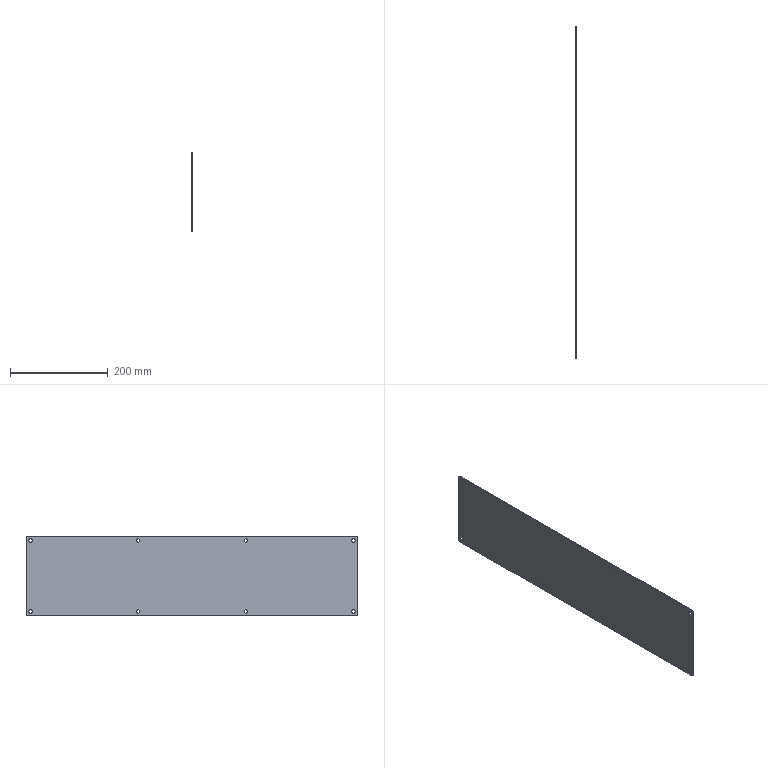Part | NX | features solid 2 | 1 solid | 26 faces | box 1.5 x 678 x 163 mm | volume 165289 mm3 | cylinder 20 | plane 6 | commonest cylinder face diameters 7 x16 8 x4
STEP:
#1=CARTESIAN_POINT('',(-1101.5,-560.,-226.5));
#2=VERTEX_POINT('',#1);
#3=CARTESIAN_POINT('',(-1100.,-560.,-226.5));
#4=VERTEX_POINT('',#3);
#5=CARTESIAN_POINT('',(-404.18,-560.,-226.5));
#6=DIRECTION('',(-1.,0.,0.));
#7=VECTOR('',#6,1000.);
#8=LINE('',#5,#7);
#9=EDGE_CURVE('',#2,#4,#8,.F.);
#10=ORIENTED_EDGE('',*,*,#9,.T.);
#11=CARTESIAN_POINT('',(-1100.,-560.,-233.5));
#12=VERTEX_POINT('',#11);
#13=CARTESIAN_POINT('',(-1100.,-560.,-230.));
#14=DIRECTION('',(-1.,0.,0.));
#15=DIRECTION('',(0.,0.,-1.));
#16=AXIS2_PLACEMENT_3D('',#13,#14,#15);
#17=CIRCLE('',#16,3.5);
#18=EDGE_CURVE('',#12,#4,#17,.T.);
#19=ORIENTED_EDGE('',*,*,#18,.F.);
#20=CARTESIAN_POINT('',(-1101.5,-560.,-233.5));
#21=VERTEX_POINT('',#20);
#22=CARTESIAN_POINT('',(-404.18,-560.,-233.5));
#23=DIRECTION('',(-1.,0.,0.));
#24=VECTOR('',#23,1000.);
#25=LINE('',#22,#24);
#26=EDGE_CURVE('',#12,#21,#25,.T.);
#27=ORIENTED_EDGE('',*,*,#26,.T.);
#28=CARTESIAN_POINT('',(-1101.5,-560.,-230.));
#29=DIRECTION('',(-1.,0.,0.));
#30=DIRECTION('',(0.,-1.,0.));
#31=AXIS2_PLACEMENT_3D('',#28,#29,#30);
#32=CIRCLE('',#31,3.5);
#33=EDGE_CURVE('',#21,#2,#32,.T.);
#34=ORIENTED_EDGE('',*,*,#33,.T.);
#35=EDGE_LOOP('',(#10,#19,#27,#34));
#36=FACE_BOUND('',#35,.T.);
#37=CARTESIAN_POINT('',(-404.18,-560.,-230.));
#38=DIRECTION('',(-1.,0.,0.));
#39=DIRECTION('',(0.,0.,-1.));
#40=AXIS2_PLACEMENT_3D('',#37,#38,#39);
#41=CYLINDRICAL_SURFACE('',#40,3.5);
#42=ADVANCED_FACE('',(#36),#41,.F.);
#43=CARTESIAN_POINT('',(-1100.,-340.,-226.5));
#44=VERTEX_POINT('',#43);
#45=CARTESIAN_POINT('',(-1101.5,-340.,-226.5));
#46=VERTEX_POINT('',#45);
#47=CARTESIAN_POINT('',(-404.18,-340.,-226.5));
#48=DIRECTION('',(-1.,0.,0.));
#49=VECTOR('',#48,1000.);
#50=LINE('',#47,#49);
#51=EDGE_CURVE('',#44,#46,#50,.T.);
#52=ORIENTED_EDGE('',*,*,#51,.F.);
#53=CARTESIAN_POINT('',(-1100.,-340.,-233.5));
#54=VERTEX_POINT('',#53);
#55=CARTESIAN_POINT('',(-1100.,-340.,-230.));
#56=DIRECTION('',(-1.,0.,0.));
#57=DIRECTION('',(0.,0.,-1.));
#58=AXIS2_PLACEMENT_3D('',#55,#56,#57);
#59=CIRCLE('',#58,3.5);
#60=EDGE_CURVE('',#54,#44,#59,.T.);
#61=ORIENTED_EDGE('',*,*,#60,.F.);
#62=CARTESIAN_POINT('',(-1101.5,-340.,-233.5));
#63=VERTEX_POINT('',#62);
#64=CARTESIAN_POINT('',(-404.18,-340.,-233.5));
#65=DIRECTION('',(-1.,0.,0.));
#66=VECTOR('',#65,1000.);
#67=LINE('',#64,#66);
#68=EDGE_CURVE('',#63,#54,#67,.F.);
#69=ORIENTED_EDGE('',*,*,#68,.F.);
#70=CARTESIAN_POINT('',(-1101.5,-340.,-230.));
#71=DIRECTION('',(-1.,0.,0.));
#72=DIRECTION('',(0.,-1.,0.));
#73=AXIS2_PLACEMENT_3D('',#70,#71,#72);
#74=CIRCLE('',#73,3.5);
#75=EDGE_CURVE('',#63,#46,#74,.T.);
#76=ORIENTED_EDGE('',*,*,#75,.T.);
#77=EDGE_LOOP('',(#52,#61,#69,#76));
#78=FACE_BOUND('',#77,.T.);
#79=CARTESIAN_POINT('',(-404.18,-340.,-230.));
#80=DIRECTION('',(-1.,0.,0.));
#81=DIRECTION('',(0.,0.,-1.));
#82=AXIS2_PLACEMENT_3D('',#79,#80,#81);
#83=CYLINDRICAL_SURFACE('',#82,3.5);
#84=ADVANCED_FACE('',(#78),#83,.F.);
#85=CARTESIAN_POINT('',(-1101.5,-340.,-81.5));
#86=VERTEX_POINT('',#85);
#87=CARTESIAN_POINT('',(-1100.,-340.,-81.5));
#88=VERTEX_POINT('',#87);
#89=CARTESIAN_POINT('',(-404.18,-340.,-81.5));
#90=DIRECTION('',(-1.,0.,0.));
#91=VECTOR('',#90,1000.);
#92=LINE('',#89,#91);
#93=EDGE_CURVE('',#86,#88,#92,.F.);
#94=ORIENTED_EDGE('',*,*,#93,.T.);
#95=CARTESIAN_POINT('',(-1100.,-340.,-88.5));
#96=VERTEX_POINT('',#95);
#97=CARTESIAN_POINT('',(-1100.,-340.,-85.));
#98=DIRECTION('',(-1.,0.,0.));
#99=DIRECTION('',(0.,0.,-1.));
#100=AXIS2_PLACEMENT_3D('',#97,#98,#99);
#101=CIRCLE('',#100,3.5);
#102=EDGE_CURVE('',#96,#88,#101,.T.);
#103=ORIENTED_EDGE('',*,*,#102,.F.);
#104=CARTESIAN_POINT('',(-1101.5,-340.,-88.5));
#105=VERTEX_POINT('',#104);
#106=CARTESIAN_POINT('',(-404.18,-340.,-88.5));
#107=DIRECTION('',(-1.,0.,0.));
#108=VECTOR('',#107,1000.);
#109=LINE('',#106,#108);
#110=EDGE_CURVE('',#96,#105,#109,.T.);
#111=ORIENTED_EDGE('',*,*,#110,.T.);
#112=CARTESIAN_POINT('',(-1101.5,-340.,-85.));
#113=DIRECTION('',(-1.,0.,0.));
#114=DIRECTION('',(0.,-1.,0.));
#115=AXIS2_PLACEMENT_3D('',#112,#113,#114);
#116=CIRCLE('',#115,3.5);
#117=EDGE_CURVE('',#105,#86,#116,.T.);
#118=ORIENTED_EDGE('',*,*,#117,.T.);
#119=EDGE_LOOP('',(#94,#103,#111,#118));
#120=FACE_BOUND('',#119,.T.);
#121=CARTESIAN_POINT('',(-404.18,-340.,-85.));
#122=DIRECTION('',(-1.,0.,0.));
#123=DIRECTION('',(0.,0.,-1.));
#124=AXIS2_PLACEMENT_3D('',#121,#122,#123);
#125=CYLINDRICAL_SURFACE('',#124,3.5);
#126=ADVANCED_FACE('',(#120),#125,.F.);
#127=CARTESIAN_POINT('',(-1100.,-560.,-81.5));
#128=VERTEX_POINT('',#127);
#129=CARTESIAN_POINT('',(-1101.5,-560.,-81.5));
#130=VERTEX_POINT('',#129);
#131=CARTESIAN_POINT('',(-404.18,-560.,-81.5));
#132=DIRECTION('',(-1.,0.,0.));
#133=VECTOR('',#132,1000.);
#134=LINE('',#131,#133);
#135=EDGE_CURVE('',#128,#130,#134,.T.);
#136=ORIENTED_EDGE('',*,*,#135,.F.);
#137=CARTESIAN_POINT('',(-1100.,-560.,-88.5));
#138=VERTEX_POINT('',#137);
#139=CARTESIAN_POINT('',(-1100.,-560.,-85.));
#140=DIRECTION('',(-1.,0.,0.));
#141=DIRECTION('',(0.,0.,-1.));
#142=AXIS2_PLACEMENT_3D('',#139,#140,#141);
#143=CIRCLE('',#142,3.5);
#144=EDGE_CURVE('',#138,#128,#143,.T.);
#145=ORIENTED_EDGE('',*,*,#144,.F.);
#146=CARTESIAN_POINT('',(-1101.5,-560.,-88.5));
#147=VERTEX_POINT('',#146);
#148=CARTESIAN_POINT('',(-404.18,-560.,-88.5));
#149=DIRECTION('',(-1.,0.,0.));
#150=VECTOR('',#149,1000.);
#151=LINE('',#148,#150);
#152=EDGE_CURVE('',#147,#138,#151,.F.);
#153=ORIENTED_EDGE('',*,*,#152,.F.);
#154=CARTESIAN_POINT('',(-1101.5,-560.,-85.));
#155=DIRECTION('',(-1.,0.,0.));
#156=DIRECTION('',(0.,-1.,0.));
#157=AXIS2_PLACEMENT_3D('',#154,#155,#156);
#158=CIRCLE('',#157,3.5);
#159=EDGE_CURVE('',#147,#130,#158,.T.);
#160=ORIENTED_EDGE('',*,*,#159,.T.);
#161=EDGE_LOOP('',(#136,#145,#153,#160));
#162=FACE_BOUND('',#161,.T.);
#163=CARTESIAN_POINT('',(-404.18,-560.,-85.));
#164=DIRECTION('',(-1.,0.,0.));
#165=DIRECTION('',(0.,0.,-1.));
#166=AXIS2_PLACEMENT_3D('',#163,#164,#165);
#167=CYLINDRICAL_SURFACE('',#166,3.5);
#168=ADVANCED_FACE('',(#162),#167,.F.);
#169=CARTESIAN_POINT('',(-1100.,-780.,-226.5));
#170=VERTEX_POINT('',#169);
#171=CARTESIAN_POINT('',(-1101.5,-780.,-226.5));
#172=VERTEX_POINT('',#171);
#173=CARTESIAN_POINT('',(-404.18,-780.,-226.5));
#174=DIRECTION('',(-1.,0.,0.));
#175=VECTOR('',#174,1000.);
#176=LINE('',#173,#175);
#177=EDGE_CURVE('',#170,#172,#176,.T.);
#178=ORIENTED_EDGE('',*,*,#177,.F.);
#179=CARTESIAN_POINT('',(-1100.,-780.,-233.5));
#180=VERTEX_POINT('',#179);
#181=CARTESIAN_POINT('',(-1100.,-780.,-230.));
#182=DIRECTION('',(-1.,0.,0.));
#183=DIRECTION('',(0.,0.,-1.));
#184=AXIS2_PLACEMENT_3D('',#181,#182,#183);
#185=CIRCLE('',#184,3.5);
#186=EDGE_CURVE('',#180,#170,#185,.T.);
#187=ORIENTED_EDGE('',*,*,#186,.F.);
#188=CARTESIAN_POINT('',(-1101.5,-780.,-233.5));
#189=VERTEX_POINT('',#188);
#190=CARTESIAN_POINT('',(-404.18,-780.,-233.5));
#191=DIRECTION('',(-1.,0.,0.));
#192=VECTOR('',#191,1000.);
#193=LINE('',#190,#192);
#194=EDGE_CURVE('',#189,#180,#193,.F.);
#195=ORIENTED_EDGE('',*,*,#194,.F.);
#196=CARTESIAN_POINT('',(-1101.5,-780.,-230.));
#197=DIRECTION('',(-1.,0.,0.));
#198=DIRECTION('',(0.,-1.,0.));
#199=AXIS2_PLACEMENT_3D('',#196,#197,#198);
#200=CIRCLE('',#199,3.5);
#201=EDGE_CURVE('',#189,#172,#200,.T.);
#202=ORIENTED_EDGE('',*,*,#201,.T.);
#203=EDGE_LOOP('',(#178,#187,#195,#202));
#204=FACE_BOUND('',#203,.T.);
#205=CARTESIAN_POINT('',(-404.18,-780.,-230.));
#206=DIRECTION('',(-1.,0.,0.));
#207=DIRECTION('',(0.,0.,-1.));
#208=AXIS2_PLACEMENT_3D('',#205,#206,#207);
#209=CYLINDRICAL_SURFACE('',#208,3.5);
#210=ADVANCED_FACE('',(#204),#209,.F.);
#211=CARTESIAN_POINT('',(-1100.,-1000.,-226.5));
#212=VERTEX_POINT('',#211);
#213=CARTESIAN_POINT('',(-1101.5,-1000.,-226.5));
#214=VERTEX_POINT('',#213);
#215=CARTESIAN_POINT('',(-404.18,-1000.,-226.5));
#216=DIRECTION('',(-1.,0.,0.));
#217=VECTOR('',#216,1000.);
#218=LINE('',#215,#217);
#219=EDGE_CURVE('',#212,#214,#218,.T.);
#220=ORIENTED_EDGE('',*,*,#219,.F.);
#221=CARTESIAN_POINT('',(-1100.,-1000.,-233.5));
#222=VERTEX_POINT('',#221);
#223=CARTESIAN_POINT('',(-1100.,-1000.,-230.));
#224=DIRECTION('',(-1.,0.,0.));
#225=DIRECTION('',(0.,0.,-1.));
#226=AXIS2_PLACEMENT_3D('',#223,#224,#225);
#227=CIRCLE('',#226,3.5);
#228=EDGE_CURVE('',#222,#212,#227,.T.);
#229=ORIENTED_EDGE('',*,*,#228,.F.);
#230=CARTESIAN_POINT('',(-1101.5,-1000.,-233.5));
#231=VERTEX_POINT('',#230);
#232=CARTESIAN_POINT('',(-404.18,-1000.,-233.5));
#233=DIRECTION('',(-1.,0.,0.));
#234=VECTOR('',#233,1000.);
#235=LINE('',#232,#234);
#236=EDGE_CURVE('',#231,#222,#235,.F.);
#237=ORIENTED_EDGE('',*,*,#236,.F.);
#238=CARTESIAN_POINT('',(-1101.5,-1000.,-230.));
#239=DIRECTION('',(-1.,0.,0.));
#240=DIRECTION('',(0.,-1.,0.));
#241=AXIS2_PLACEMENT_3D('',#238,#239,#240);
#242=CIRCLE('',#241,3.5);
#243=EDGE_CURVE('',#231,#214,#242,.T.);
#244=ORIENTED_EDGE('',*,*,#243,.T.);
#245=EDGE_LOOP('',(#220,#229,#237,#244));
#246=FACE_BOUND('',#245,.T.);
#247=CARTESIAN_POINT('',(-404.18,-1000.,-230.));
#248=DIRECTION('',(-1.,0.,0.));
#249=DIRECTION('',(0.,0.,-1.));
#250=AXIS2_PLACEMENT_3D('',#247,#248,#249);
#251=CYLINDRICAL_SURFACE('',#250,3.5);
#252=ADVANCED_FACE('',(#246),#251,.F.);
#253=CARTESIAN_POINT('',(-1101.5,-780.,-81.5));
#254=VERTEX_POINT('',#253);
#255=CARTESIAN_POINT('',(-1100.,-780.,-81.5));
#256=VERTEX_POINT('',#255);
#257=CARTESIAN_POINT('',(-404.18,-780.,-81.5));
#258=DIRECTION('',(-1.,0.,0.));
#259=VECTOR('',#258,1000.);
#260=LINE('',#257,#259);
#261=EDGE_CURVE('',#254,#256,#260,.F.);
#262=ORIENTED_EDGE('',*,*,#261,.T.);
#263=CARTESIAN_POINT('',(-1100.,-780.,-88.5));
#264=VERTEX_POINT('',#263);
#265=CARTESIAN_POINT('',(-1100.,-780.,-85.));
#266=DIRECTION('',(-1.,0.,0.));
#267=DIRECTION('',(0.,0.,-1.));
#268=AXIS2_PLACEMENT_3D('',#265,#266,#267);
#269=CIRCLE('',#268,3.5);
#270=EDGE_CURVE('',#264,#256,#269,.T.);
#271=ORIENTED_EDGE('',*,*,#270,.F.);
#272=CARTESIAN_POINT('',(-1101.5,-780.,-88.5));
#273=VERTEX_POINT('',#272);
#274=CARTESIAN_POINT('',(-404.18,-780.,-88.5));
#275=DIRECTION('',(-1.,0.,0.));
#276=VECTOR('',#275,1000.);
#277=LINE('',#274,#276);
#278=EDGE_CURVE('',#264,#273,#277,.T.);
#279=ORIENTED_EDGE('',*,*,#278,.T.);
#280=CARTESIAN_POINT('',(-1101.5,-780.,-85.));
#281=DIRECTION('',(-1.,0.,0.));
#282=DIRECTION('',(0.,-1.,0.));
#283=AXIS2_PLACEMENT_3D('',#280,#281,#282);
#284=CIRCLE('',#283,3.5);
#285=EDGE_CURVE('',#273,#254,#284,.T.);
#286=ORIENTED_EDGE('',*,*,#285,.T.);
#287=EDGE_LOOP('',(#262,#271,#279,#286));
#288=FACE_BOUND('',#287,.T.);
#289=CARTESIAN_POINT('',(-404.18,-780.,-85.));
#290=DIRECTION('',(-1.,0.,0.));
#291=DIRECTION('',(0.,0.,-1.));
#292=AXIS2_PLACEMENT_3D('',#289,#290,#291);
#293=CYLINDRICAL_SURFACE('',#292,3.5);
#294=ADVANCED_FACE('',(#288),#293,.F.);
#295=CARTESIAN_POINT('',(-1100.,-1000.,-81.5));
#296=VERTEX_POINT('',#295);
#297=CARTESIAN_POINT('',(-1101.5,-1000.,-81.5));
#298=VERTEX_POINT('',#297);
#299=CARTESIAN_POINT('',(-404.18,-1000.,-81.5));
#300=DIRECTION('',(-1.,0.,0.));
#301=VECTOR('',#300,1000.);
#302=LINE('',#299,#301);
#303=EDGE_CURVE('',#296,#298,#302,.T.);
#304=ORIENTED_EDGE('',*,*,#303,.F.);
#305=CARTESIAN_POINT('',(-1100.,-1000.,-88.5));
#306=VERTEX_POINT('',#305);
#307=CARTESIAN_POINT('',(-1100.,-1000.,-85.));
#308=DIRECTION('',(-1.,0.,0.));
#309=DIRECTION('',(0.,0.,-1.));
#310=AXIS2_PLACEMENT_3D('',#307,#308,#309);
#311=CIRCLE('',#310,3.5);
#312=EDGE_CURVE('',#306,#296,#311,.T.);
#313=ORIENTED_EDGE('',*,*,#312,.F.);
#314=CARTESIAN_POINT('',(-1101.5,-1000.,-88.5));
#315=VERTEX_POINT('',#314);
#316=CARTESIAN_POINT('',(-404.18,-1000.,-88.5));
#317=DIRECTION('',(-1.,0.,0.));
#318=VECTOR('',#317,1000.);
#319=LINE('',#316,#318);
#320=EDGE_CURVE('',#315,#306,#319,.F.);
#321=ORIENTED_EDGE('',*,*,#320,.F.);
#322=CARTESIAN_POINT('',(-1101.5,-1000.,-85.));
#323=DIRECTION('',(-1.,0.,0.));
#324=DIRECTION('',(0.,-1.,0.));
#325=AXIS2_PLACEMENT_3D('',#322,#323,#324);
#326=CIRCLE('',#325,3.5);
#327=EDGE_CURVE('',#315,#298,#326,.T.);
#328=ORIENTED_EDGE('',*,*,#327,.T.);
#329=EDGE_LOOP('',(#304,#313,#321,#328));
#330=FACE_BOUND('',#329,.T.);
#331=CARTESIAN_POINT('',(-404.18,-1000.,-85.));
#332=DIRECTION('',(-1.,0.,0.));
#333=DIRECTION('',(0.,0.,-1.));
#334=AXIS2_PLACEMENT_3D('',#331,#332,#333);
#335=CYLINDRICAL_SURFACE('',#334,3.5);
#336=ADVANCED_FACE('',(#330),#335,.F.);
#337=ORIENTED_EDGE('',*,*,#312,.T.);
#338=CARTESIAN_POINT('',(-1100.,-1000.,-85.));
#339=DIRECTION('',(-1.,0.,0.));
#340=DIRECTION('',(0.,0.,-1.));
#341=AXIS2_PLACEMENT_3D('',#338,#339,#340);
#342=CIRCLE('',#341,3.5);
#343=EDGE_CURVE('',#296,#306,#342,.T.);
#344=ORIENTED_EDGE('',*,*,#343,.T.);
#345=EDGE_LOOP('',(#337,#344));
#346=FACE_BOUND('',#345,.T.);
#347=ORIENTED_EDGE('',*,*,#270,.T.);
#348=CARTESIAN_POINT('',(-1100.,-780.,-85.));
#349=DIRECTION('',(-1.,0.,0.));
#350=DIRECTION('',(0.,0.,-1.));
#351=AXIS2_PLACEMENT_3D('',#348,#349,#350);
#352=CIRCLE('',#351,3.5);
#353=EDGE_CURVE('',#256,#264,#352,.T.);
#354=ORIENTED_EDGE('',*,*,#353,.T.);
#355=EDGE_LOOP('',(#347,#354));
#356=FACE_BOUND('',#355,.T.);
#357=ORIENTED_EDGE('',*,*,#228,.T.);
#358=CARTESIAN_POINT('',(-1100.,-1000.,-230.));
#359=DIRECTION('',(-1.,0.,0.));
#360=DIRECTION('',(0.,0.,-1.));
#361=AXIS2_PLACEMENT_3D('',#358,#359,#360);
#362=CIRCLE('',#361,3.5);
#363=EDGE_CURVE('',#212,#222,#362,.T.);
#364=ORIENTED_EDGE('',*,*,#363,.T.);
#365=EDGE_LOOP('',(#357,#364));
#366=FACE_BOUND('',#365,.T.);
#367=ORIENTED_EDGE('',*,*,#186,.T.);
#368=CARTESIAN_POINT('',(-1100.,-780.,-230.));
#369=DIRECTION('',(-1.,0.,0.));
#370=DIRECTION('',(0.,0.,-1.));
#371=AXIS2_PLACEMENT_3D('',#368,#369,#370);
#372=CIRCLE('',#371,3.5);
#373=EDGE_CURVE('',#170,#180,#372,.T.);
#374=ORIENTED_EDGE('',*,*,#373,.T.);
#375=EDGE_LOOP('',(#367,#374));
#376=FACE_BOUND('',#375,.T.);
#377=ORIENTED_EDGE('',*,*,#144,.T.);
#378=CARTESIAN_POINT('',(-1100.,-560.,-85.));
#379=DIRECTION('',(-1.,0.,0.));
#380=DIRECTION('',(0.,0.,-1.));
#381=AXIS2_PLACEMENT_3D('',#378,#379,#380);
#382=CIRCLE('',#381,3.5);
#383=EDGE_CURVE('',#128,#138,#382,.T.);
#384=ORIENTED_EDGE('',*,*,#383,.T.);
#385=EDGE_LOOP('',(#377,#384));
#386=FACE_BOUND('',#385,.T.);
#387=ORIENTED_EDGE('',*,*,#102,.T.);
#388=CARTESIAN_POINT('',(-1100.,-340.,-85.));
#389=DIRECTION('',(-1.,0.,0.));
#390=DIRECTION('',(0.,0.,-1.));
#391=AXIS2_PLACEMENT_3D('',#388,#389,#390);
#392=CIRCLE('',#391,3.5);
#393=EDGE_CURVE('',#88,#96,#392,.T.);
#394=ORIENTED_EDGE('',*,*,#393,.T.);
#395=EDGE_LOOP('',(#387,#394));
#396=FACE_BOUND('',#395,.T.);
#397=ORIENTED_EDGE('',*,*,#60,.T.);
#398=CARTESIAN_POINT('',(-1100.,-340.,-230.));
#399=DIRECTION('',(-1.,0.,0.));
#400=DIRECTION('',(0.,0.,-1.));
#401=AXIS2_PLACEMENT_3D('',#398,#399,#400);
#402=CIRCLE('',#401,3.5);
#403=EDGE_CURVE('',#44,#54,#402,.T.);
#404=ORIENTED_EDGE('',*,*,#403,.T.);
#405=EDGE_LOOP('',(#397,#404));
#406=FACE_BOUND('',#405,.T.);
#407=ORIENTED_EDGE('',*,*,#18,.T.);
#408=CARTESIAN_POINT('',(-1100.,-560.,-230.));
#409=DIRECTION('',(-1.,0.,0.));
#410=DIRECTION('',(0.,0.,-1.));
#411=AXIS2_PLACEMENT_3D('',#408,#409,#410);
#412=CIRCLE('',#411,3.5);
#413=EDGE_CURVE('',#4,#12,#412,.T.);
#414=ORIENTED_EDGE('',*,*,#413,.T.);
#415=EDGE_LOOP('',(#407,#414));
#416=FACE_BOUND('',#415,.T.);
#417=CARTESIAN_POINT('',(-1100.,-335.,-76.));
#418=VERTEX_POINT('',#417);
#419=CARTESIAN_POINT('',(-1100.,-331.,-80.));
#420=VERTEX_POINT('',#419);
#421=CARTESIAN_POINT('',(-1100.,-335.,-80.));
#422=DIRECTION('',(-1.,0.,0.));
#423=DIRECTION('',(0.,-1.,0.));
#424=AXIS2_PLACEMENT_3D('',#421,#422,#423);
#425=CIRCLE('',#424,4.);
#426=EDGE_CURVE('',#418,#420,#425,.T.);
#427=ORIENTED_EDGE('',*,*,#426,.F.);
#428=CARTESIAN_POINT('',(-1100.,-1005.,-76.));
#429=VERTEX_POINT('',#428);
#430=CARTESIAN_POINT('',(-1100.,-1005.,-76.));
#431=DIRECTION('',(0.,1.,0.));
#432=VECTOR('',#431,1000.);
#433=LINE('',#430,#432);
#434=EDGE_CURVE('',#429,#418,#433,.T.);
#435=ORIENTED_EDGE('',*,*,#434,.F.);
#436=CARTESIAN_POINT('',(-1100.,-1009.,-80.));
#437=VERTEX_POINT('',#436);
#438=CARTESIAN_POINT('',(-1100.,-1005.,-80.));
#439=DIRECTION('',(-1.,0.,0.));
#440=DIRECTION('',(0.,-1.,0.));
#441=AXIS2_PLACEMENT_3D('',#438,#439,#440);
#442=CIRCLE('',#441,4.);
#443=EDGE_CURVE('',#437,#429,#442,.T.);
#444=ORIENTED_EDGE('',*,*,#443,.F.);
#445=CARTESIAN_POINT('',(-1100.,-1009.,-235.));
#446=VERTEX_POINT('',#445);
#447=CARTESIAN_POINT('',(-1100.,-1009.,-235.));
#448=DIRECTION('',(0.,0.,1.));
#449=VECTOR('',#448,1000.);
#450=LINE('',#447,#449);
#451=EDGE_CURVE('',#446,#437,#450,.T.);
#452=ORIENTED_EDGE('',*,*,#451,.F.);
#453=CARTESIAN_POINT('',(-1100.,-1005.,-239.));
#454=VERTEX_POINT('',#453);
#455=CARTESIAN_POINT('',(-1100.,-1005.,-235.));
#456=DIRECTION('',(-1.,0.,0.));
#457=DIRECTION('',(0.,1.,0.));
#458=AXIS2_PLACEMENT_3D('',#455,#456,#457);
#459=CIRCLE('',#458,4.);
#460=EDGE_CURVE('',#454,#446,#459,.T.);
#461=ORIENTED_EDGE('',*,*,#460,.F.);
#462=CARTESIAN_POINT('',(-1100.,-335.,-239.));
#463=VERTEX_POINT('',#462);
#464=CARTESIAN_POINT('',(-1100.,-335.,-239.));
#465=DIRECTION('',(0.,-1.,0.));
#466=VECTOR('',#465,1000.);
#467=LINE('',#464,#466);
#468=EDGE_CURVE('',#463,#454,#467,.T.);
#469=ORIENTED_EDGE('',*,*,#468,.F.);
#470=CARTESIAN_POINT('',(-1100.,-331.,-235.));
#471=VERTEX_POINT('',#470);
#472=CARTESIAN_POINT('',(-1100.,-335.,-235.));
#473=DIRECTION('',(-1.,0.,0.));
#474=DIRECTION('',(0.,-1.,0.));
#475=AXIS2_PLACEMENT_3D('',#472,#473,#474);
#476=CIRCLE('',#475,4.);
#477=EDGE_CURVE('',#471,#463,#476,.T.);
#478=ORIENTED_EDGE('',*,*,#477,.F.);
#479=CARTESIAN_POINT('',(-1100.,-331.,-80.));
#480=DIRECTION('',(0.,0.,-1.));
#481=VECTOR('',#480,1000.);
#482=LINE('',#479,#481);
#483=EDGE_CURVE('',#420,#471,#482,.T.);
#484=ORIENTED_EDGE('',*,*,#483,.F.);
#485=EDGE_LOOP('',(#427,#435,#444,#452,#461,#469,#478,#484));
#486=FACE_BOUND('',#485,.T.);
#487=CARTESIAN_POINT('',(-1100.,-335.,-80.));
#488=DIRECTION('',(-1.,0.,0.));
#489=DIRECTION('',(0.,0.,1.));
#490=AXIS2_PLACEMENT_3D('',#487,#488,#489);
#491=PLANE('',#490);
#492=ADVANCED_FACE('',(#346,#356,#366,#376,#386,#396,#406,#416,#486),#491,.F.);
#493=ORIENTED_EDGE('',*,*,#327,.F.);
#494=CARTESIAN_POINT('',(-1101.5,-1000.,-85.));
#495=DIRECTION('',(-1.,0.,0.));
#496=DIRECTION('',(0.,-1.,0.));
#497=AXIS2_PLACEMENT_3D('',#494,#495,#496);
#498=CIRCLE('',#497,3.5);
#499=EDGE_CURVE('',#298,#315,#498,.T.);
#500=ORIENTED_EDGE('',*,*,#499,.F.);
#501=EDGE_LOOP('',(#493,#500));
#502=FACE_BOUND('',#501,.T.);
#503=ORIENTED_EDGE('',*,*,#285,.F.);
#504=CARTESIAN_POINT('',(-1101.5,-780.,-85.));
#505=DIRECTION('',(-1.,0.,0.));
#506=DIRECTION('',(0.,-1.,0.));
#507=AXIS2_PLACEMENT_3D('',#504,#505,#506);
#508=CIRCLE('',#507,3.5);
#509=EDGE_CURVE('',#254,#273,#508,.T.);
#510=ORIENTED_EDGE('',*,*,#509,.F.);
#511=EDGE_LOOP('',(#503,#510));
#512=FACE_BOUND('',#511,.T.);
#513=ORIENTED_EDGE('',*,*,#243,.F.);
#514=CARTESIAN_POINT('',(-1101.5,-1000.,-230.));
#515=DIRECTION('',(-1.,0.,0.));
#516=DIRECTION('',(0.,-1.,0.));
#517=AXIS2_PLACEMENT_3D('',#514,#515,#516);
#518=CIRCLE('',#517,3.5);
#519=EDGE_CURVE('',#214,#231,#518,.T.);
#520=ORIENTED_EDGE('',*,*,#519,.F.);
#521=EDGE_LOOP('',(#513,#520));
#522=FACE_BOUND('',#521,.T.);
#523=ORIENTED_EDGE('',*,*,#201,.F.);
#524=CARTESIAN_POINT('',(-1101.5,-780.,-230.));
#525=DIRECTION('',(-1.,0.,0.));
#526=DIRECTION('',(0.,-1.,0.));
#527=AXIS2_PLACEMENT_3D('',#524,#525,#526);
#528=CIRCLE('',#527,3.5);
#529=EDGE_CURVE('',#172,#189,#528,.T.);
#530=ORIENTED_EDGE('',*,*,#529,.F.);
#531=EDGE_LOOP('',(#523,#530));
#532=FACE_BOUND('',#531,.T.);
#533=ORIENTED_EDGE('',*,*,#159,.F.);
#534=CARTESIAN_POINT('',(-1101.5,-560.,-85.));
#535=DIRECTION('',(-1.,0.,0.));
#536=DIRECTION('',(0.,-1.,0.));
#537=AXIS2_PLACEMENT_3D('',#534,#535,#536);
#538=CIRCLE('',#537,3.5);
#539=EDGE_CURVE('',#130,#147,#538,.T.);
#540=ORIENTED_EDGE('',*,*,#539,.F.);
#541=EDGE_LOOP('',(#533,#540));
#542=FACE_BOUND('',#541,.T.);
#543=ORIENTED_EDGE('',*,*,#117,.F.);
#544=CARTESIAN_POINT('',(-1101.5,-340.,-85.));
#545=DIRECTION('',(-1.,0.,0.));
#546=DIRECTION('',(0.,-1.,0.));
#547=AXIS2_PLACEMENT_3D('',#544,#545,#546);
#548=CIRCLE('',#547,3.5);
#549=EDGE_CURVE('',#86,#105,#548,.T.);
#550=ORIENTED_EDGE('',*,*,#549,.F.);
#551=EDGE_LOOP('',(#543,#550));
#552=FACE_BOUND('',#551,.T.);
#553=ORIENTED_EDGE('',*,*,#75,.F.);
#554=CARTESIAN_POINT('',(-1101.5,-340.,-230.));
#555=DIRECTION('',(-1.,0.,0.));
#556=DIRECTION('',(0.,-1.,0.));
#557=AXIS2_PLACEMENT_3D('',#554,#555,#556);
#558=CIRCLE('',#557,3.5);
#559=EDGE_CURVE('',#46,#63,#558,.T.);
#560=ORIENTED_EDGE('',*,*,#559,.F.);
#561=EDGE_LOOP('',(#553,#560));
#562=FACE_BOUND('',#561,.T.);
#563=ORIENTED_EDGE('',*,*,#33,.F.);
#564=CARTESIAN_POINT('',(-1101.5,-560.,-230.));
#565=DIRECTION('',(-1.,0.,0.));
#566=DIRECTION('',(0.,-1.,0.));
#567=AXIS2_PLACEMENT_3D('',#564,#565,#566);
#568=CIRCLE('',#567,3.5);
#569=EDGE_CURVE('',#2,#21,#568,.T.);
#570=ORIENTED_EDGE('',*,*,#569,.F.);
#571=EDGE_LOOP('',(#563,#570));
#572=FACE_BOUND('',#571,.T.);
#573=CARTESIAN_POINT('',(-1101.5,-335.,-76.));
#574=VERTEX_POINT('',#573);
#575=CARTESIAN_POINT('',(-1101.5,-331.,-80.));
#576=VERTEX_POINT('',#575);
#577=CARTESIAN_POINT('',(-1101.5,-335.,-80.));
#578=DIRECTION('',(-1.,0.,0.));
#579=DIRECTION('',(0.,-1.,0.));
#580=AXIS2_PLACEMENT_3D('',#577,#578,#579);
#581=CIRCLE('',#580,4.);
#582=EDGE_CURVE('',#574,#576,#581,.T.);
#583=ORIENTED_EDGE('',*,*,#582,.T.);
#584=CARTESIAN_POINT('',(-1101.5,-331.,-235.));
#585=VERTEX_POINT('',#584);
#586=CARTESIAN_POINT('',(-1101.5,-331.,-80.));
#587=DIRECTION('',(0.,0.,-1.));
#588=VECTOR('',#587,1000.);
#589=LINE('',#586,#588);
#590=EDGE_CURVE('',#576,#585,#589,.T.);
#591=ORIENTED_EDGE('',*,*,#590,.T.);
#592=CARTESIAN_POINT('',(-1101.5,-335.,-239.));
#593=VERTEX_POINT('',#592);
#594=CARTESIAN_POINT('',(-1101.5,-335.,-235.));
#595=DIRECTION('',(-1.,0.,0.));
#596=DIRECTION('',(0.,-1.,0.));
#597=AXIS2_PLACEMENT_3D('',#594,#595,#596);
#598=CIRCLE('',#597,4.);
#599=EDGE_CURVE('',#585,#593,#598,.T.);
#600=ORIENTED_EDGE('',*,*,#599,.T.);
#601=CARTESIAN_POINT('',(-1101.5,-1005.,-239.));
#602=VERTEX_POINT('',#601);
#603=CARTESIAN_POINT('',(-1101.5,-335.,-239.));
#604=DIRECTION('',(0.,-1.,0.));
#605=VECTOR('',#604,1000.);
#606=LINE('',#603,#605);
#607=EDGE_CURVE('',#593,#602,#606,.T.);
#608=ORIENTED_EDGE('',*,*,#607,.T.);
#609=CARTESIAN_POINT('',(-1101.5,-1009.,-235.));
#610=VERTEX_POINT('',#609);
#611=CARTESIAN_POINT('',(-1101.5,-1005.,-235.));
#612=DIRECTION('',(-1.,0.,0.));
#613=DIRECTION('',(0.,1.,0.));
#614=AXIS2_PLACEMENT_3D('',#611,#612,#613);
#615=CIRCLE('',#614,4.);
#616=EDGE_CURVE('',#602,#610,#615,.T.);
#617=ORIENTED_EDGE('',*,*,#616,.T.);
#618=CARTESIAN_POINT('',(-1101.5,-1009.,-80.));
#619=VERTEX_POINT('',#618);
#620=CARTESIAN_POINT('',(-1101.5,-1009.,-235.));
#621=DIRECTION('',(0.,0.,1.));
#622=VECTOR('',#621,1000.);
#623=LINE('',#620,#622);
#624=EDGE_CURVE('',#610,#619,#623,.T.);
#625=ORIENTED_EDGE('',*,*,#624,.T.);
#626=CARTESIAN_POINT('',(-1101.5,-1005.,-76.));
#627=VERTEX_POINT('',#626);
#628=CARTESIAN_POINT('',(-1101.5,-1005.,-80.));
#629=DIRECTION('',(-1.,0.,0.));
#630=DIRECTION('',(0.,-1.,0.));
#631=AXIS2_PLACEMENT_3D('',#628,#629,#630);
#632=CIRCLE('',#631,4.);
#633=EDGE_CURVE('',#619,#627,#632,.T.);
#634=ORIENTED_EDGE('',*,*,#633,.T.);
#635=CARTESIAN_POINT('',(-1101.5,-1005.,-76.));
#636=DIRECTION('',(0.,1.,0.));
#637=VECTOR('',#636,1000.);
#638=LINE('',#635,#637);
#639=EDGE_CURVE('',#627,#574,#638,.T.);
#640=ORIENTED_EDGE('',*,*,#639,.T.);
#641=EDGE_LOOP('',(#583,#591,#600,#608,#617,#625,#634,#640));
#642=FACE_BOUND('',#641,.T.);
#643=CARTESIAN_POINT('',(-1101.5,-335.,-80.));
#644=DIRECTION('',(-1.,0.,0.));
#645=DIRECTION('',(0.,0.,1.));
#646=AXIS2_PLACEMENT_3D('',#643,#644,#645);
#647=PLANE('',#646);
#648=ADVANCED_FACE('',(#502,#512,#522,#532,#542,#552,#562,#572,#642),#647,.T.);
#649=ORIENTED_EDGE('',*,*,#434,.T.);
#650=CARTESIAN_POINT('',(-1101.5,-335.,-76.));
#651=DIRECTION('',(1.,0.,0.));
#652=VECTOR('',#651,1000.);
#653=LINE('',#650,#652);
#654=EDGE_CURVE('',#574,#418,#653,.T.);
#655=ORIENTED_EDGE('',*,*,#654,.F.);
#656=ORIENTED_EDGE('',*,*,#639,.F.);
#657=CARTESIAN_POINT('',(-1101.5,-1005.,-76.));
#658=DIRECTION('',(1.,0.,0.));
#659=VECTOR('',#658,1000.);
#660=LINE('',#657,#659);
#661=EDGE_CURVE('',#627,#429,#660,.T.);
#662=ORIENTED_EDGE('',*,*,#661,.T.);
#663=EDGE_LOOP('',(#649,#655,#656,#662));
#664=FACE_BOUND('',#663,.T.);
#665=CARTESIAN_POINT('',(-1101.5,-1005.,-76.));
#666=DIRECTION('',(0.,0.,-1.));
#667=DIRECTION('',(0.,-1.,0.));
#668=AXIS2_PLACEMENT_3D('',#665,#666,#667);
#669=PLANE('',#668);
#670=ADVANCED_FACE('',(#664),#669,.F.);
#671=ORIENTED_EDGE('',*,*,#443,.T.);
#672=ORIENTED_EDGE('',*,*,#661,.F.);
#673=ORIENTED_EDGE('',*,*,#633,.F.);
#674=CARTESIAN_POINT('',(-1101.5,-1009.,-80.));
#675=DIRECTION('',(1.,0.,0.));
#676=VECTOR('',#675,1000.);
#677=LINE('',#674,#676);
#678=EDGE_CURVE('',#619,#437,#677,.T.);
#679=ORIENTED_EDGE('',*,*,#678,.T.);
#680=EDGE_LOOP('',(#671,#672,#673,#679));
#681=FACE_BOUND('',#680,.T.);
#682=CARTESIAN_POINT('',(-1101.5,-1005.,-80.));
#683=DIRECTION('',(1.,0.,0.));
#684=DIRECTION('',(0.,0.,1.));
#685=AXIS2_PLACEMENT_3D('',#682,#683,#684);
#686=CYLINDRICAL_SURFACE('',#685,4.);
#687=ADVANCED_FACE('',(#681),#686,.T.);
#688=ORIENTED_EDGE('',*,*,#451,.T.);
#689=ORIENTED_EDGE('',*,*,#678,.F.);
#690=ORIENTED_EDGE('',*,*,#624,.F.);
#691=CARTESIAN_POINT('',(-1101.5,-1009.,-235.));
#692=DIRECTION('',(1.,0.,0.));
#693=VECTOR('',#692,1000.);
#694=LINE('',#691,#693);
#695=EDGE_CURVE('',#610,#446,#694,.T.);
#696=ORIENTED_EDGE('',*,*,#695,.T.);
#697=EDGE_LOOP('',(#688,#689,#690,#696));
#698=FACE_BOUND('',#697,.T.);
#699=CARTESIAN_POINT('',(-1101.5,-1009.,-235.));
#700=DIRECTION('',(0.,1.,0.));
#701=DIRECTION('',(0.,0.,-1.));
#702=AXIS2_PLACEMENT_3D('',#699,#700,#701);
#703=PLANE('',#702);
#704=ADVANCED_FACE('',(#698),#703,.F.);
#705=ORIENTED_EDGE('',*,*,#460,.T.);
#706=ORIENTED_EDGE('',*,*,#695,.F.);
#707=ORIENTED_EDGE('',*,*,#616,.F.);
#708=CARTESIAN_POINT('',(-1101.5,-1005.,-239.));
#709=DIRECTION('',(1.,0.,0.));
#710=VECTOR('',#709,1000.);
#711=LINE('',#708,#710);
#712=EDGE_CURVE('',#602,#454,#711,.T.);
#713=ORIENTED_EDGE('',*,*,#712,.T.);
#714=EDGE_LOOP('',(#705,#706,#707,#713));
#715=FACE_BOUND('',#714,.T.);
#716=CARTESIAN_POINT('',(-1101.5,-1005.,-235.));
#717=DIRECTION('',(1.,0.,0.));
#718=DIRECTION('',(0.,0.,1.));
#719=AXIS2_PLACEMENT_3D('',#716,#717,#718);
#720=CYLINDRICAL_SURFACE('',#719,4.);
#721=ADVANCED_FACE('',(#715),#720,.T.);
#722=ORIENTED_EDGE('',*,*,#468,.T.);
#723=ORIENTED_EDGE('',*,*,#712,.F.);
#724=ORIENTED_EDGE('',*,*,#607,.F.);
#725=CARTESIAN_POINT('',(-1101.5,-335.,-239.));
#726=DIRECTION('',(1.,0.,0.));
#727=VECTOR('',#726,1000.);
#728=LINE('',#725,#727);
#729=EDGE_CURVE('',#593,#463,#728,.T.);
#730=ORIENTED_EDGE('',*,*,#729,.T.);
#731=EDGE_LOOP('',(#722,#723,#724,#730));
#732=FACE_BOUND('',#731,.T.);
#733=CARTESIAN_POINT('',(-1101.5,-335.,-239.));
#734=DIRECTION('',(0.,0.,1.));
#735=DIRECTION('',(1.,0.,0.));
#736=AXIS2_PLACEMENT_3D('',#733,#734,#735);
#737=PLANE('',#736);
#738=ADVANCED_FACE('',(#732),#737,.F.);
#739=ORIENTED_EDGE('',*,*,#477,.T.);
#740=ORIENTED_EDGE('',*,*,#729,.F.);
#741=ORIENTED_EDGE('',*,*,#599,.F.);
#742=CARTESIAN_POINT('',(-1101.5,-331.,-235.));
#743=DIRECTION('',(1.,0.,0.));
#744=VECTOR('',#743,1000.);
#745=LINE('',#742,#744);
#746=EDGE_CURVE('',#585,#471,#745,.T.);
#747=ORIENTED_EDGE('',*,*,#746,.T.);
#748=EDGE_LOOP('',(#739,#740,#741,#747));
#749=FACE_BOUND('',#748,.T.);
#750=CARTESIAN_POINT('',(-1101.5,-335.,-235.));
#751=DIRECTION('',(1.,0.,0.));
#752=DIRECTION('',(0.,0.,1.));
#753=AXIS2_PLACEMENT_3D('',#750,#751,#752);
#754=CYLINDRICAL_SURFACE('',#753,4.);
#755=ADVANCED_FACE('',(#749),#754,.T.);
#756=ORIENTED_EDGE('',*,*,#483,.T.);
#757=ORIENTED_EDGE('',*,*,#746,.F.);
#758=ORIENTED_EDGE('',*,*,#590,.F.);
#759=CARTESIAN_POINT('',(-1101.5,-331.,-80.));
#760=DIRECTION('',(1.,0.,0.));
#761=VECTOR('',#760,1000.);
#762=LINE('',#759,#761);
#763=EDGE_CURVE('',#576,#420,#762,.T.);
#764=ORIENTED_EDGE('',*,*,#763,.T.);
#765=EDGE_LOOP('',(#756,#757,#758,#764));
#766=FACE_BOUND('',#765,.T.);
#767=CARTESIAN_POINT('',(-1101.5,-331.,-80.));
#768=DIRECTION('',(0.,-1.,0.));
#769=DIRECTION('',(0.,0.,-1.));
#770=AXIS2_PLACEMENT_3D('',#767,#768,#769);
#771=PLANE('',#770);
#772=ADVANCED_FACE('',(#766),#771,.F.);
#773=ORIENTED_EDGE('',*,*,#426,.T.);
#774=ORIENTED_EDGE('',*,*,#763,.F.);
#775=ORIENTED_EDGE('',*,*,#582,.F.);
#776=ORIENTED_EDGE('',*,*,#654,.T.);
#777=EDGE_LOOP('',(#773,#774,#775,#776));
#778=FACE_BOUND('',#777,.T.);
#779=CARTESIAN_POINT('',(-1101.5,-335.,-80.));
#780=DIRECTION('',(1.,0.,0.));
#781=DIRECTION('',(0.,0.,1.));
#782=AXIS2_PLACEMENT_3D('',#779,#780,#781);
#783=CYLINDRICAL_SURFACE('',#782,4.);
#784=ADVANCED_FACE('',(#778),#783,.T.);
#785=ORIENTED_EDGE('',*,*,#343,.F.);
#786=ORIENTED_EDGE('',*,*,#303,.T.);
#787=ORIENTED_EDGE('',*,*,#499,.T.);
#788=ORIENTED_EDGE('',*,*,#320,.T.);
#789=EDGE_LOOP('',(#785,#786,#787,#788));
#790=FACE_BOUND('',#789,.T.);
#791=CARTESIAN_POINT('',(-404.18,-1000.,-85.));
#792=DIRECTION('',(-1.,0.,0.));
#793=DIRECTION('',(0.,0.,-1.));
#794=AXIS2_PLACEMENT_3D('',#791,#792,#793);
#795=CYLINDRICAL_SURFACE('',#794,3.5);
#796=ADVANCED_FACE('',(#790),#795,.F.);
#797=ORIENTED_EDGE('',*,*,#353,.F.);
#798=ORIENTED_EDGE('',*,*,#261,.F.);
#799=ORIENTED_EDGE('',*,*,#509,.T.);
#800=ORIENTED_EDGE('',*,*,#278,.F.);
#801=EDGE_LOOP('',(#797,#798,#799,#800));
#802=FACE_BOUND('',#801,.T.);
#803=CARTESIAN_POINT('',(-404.18,-780.,-85.));
#804=DIRECTION('',(-1.,0.,0.));
#805=DIRECTION('',(0.,0.,-1.));
#806=AXIS2_PLACEMENT_3D('',#803,#804,#805);
#807=CYLINDRICAL_SURFACE('',#806,3.5);
#808=ADVANCED_FACE('',(#802),#807,.F.);
#809=ORIENTED_EDGE('',*,*,#363,.F.);
#810=ORIENTED_EDGE('',*,*,#219,.T.);
#811=ORIENTED_EDGE('',*,*,#519,.T.);
#812=ORIENTED_EDGE('',*,*,#236,.T.);
#813=EDGE_LOOP('',(#809,#810,#811,#812));
#814=FACE_BOUND('',#813,.T.);
#815=CARTESIAN_POINT('',(-404.18,-1000.,-230.));
#816=DIRECTION('',(-1.,0.,0.));
#817=DIRECTION('',(0.,0.,-1.));
#818=AXIS2_PLACEMENT_3D('',#815,#816,#817);
#819=CYLINDRICAL_SURFACE('',#818,3.5);
#820=ADVANCED_FACE('',(#814),#819,.F.);
#821=ORIENTED_EDGE('',*,*,#373,.F.);
#822=ORIENTED_EDGE('',*,*,#177,.T.);
#823=ORIENTED_EDGE('',*,*,#529,.T.);
#824=ORIENTED_EDGE('',*,*,#194,.T.);
#825=EDGE_LOOP('',(#821,#822,#823,#824));
#826=FACE_BOUND('',#825,.T.);
#827=CARTESIAN_POINT('',(-404.18,-780.,-230.));
#828=DIRECTION('',(-1.,0.,0.));
#829=DIRECTION('',(0.,0.,-1.));
#830=AXIS2_PLACEMENT_3D('',#827,#828,#829);
#831=CYLINDRICAL_SURFACE('',#830,3.5);
#832=ADVANCED_FACE('',(#826),#831,.F.);
#833=ORIENTED_EDGE('',*,*,#383,.F.);
#834=ORIENTED_EDGE('',*,*,#135,.T.);
#835=ORIENTED_EDGE('',*,*,#539,.T.);
#836=ORIENTED_EDGE('',*,*,#152,.T.);
#837=EDGE_LOOP('',(#833,#834,#835,#836));
#838=FACE_BOUND('',#837,.T.);
#839=CARTESIAN_POINT('',(-404.18,-560.,-85.));
#840=DIRECTION('',(-1.,0.,0.));
#841=DIRECTION('',(0.,0.,-1.));
#842=AXIS2_PLACEMENT_3D('',#839,#840,#841);
#843=CYLINDRICAL_SURFACE('',#842,3.5);
#844=ADVANCED_FACE('',(#838),#843,.F.);
#845=ORIENTED_EDGE('',*,*,#393,.F.);
#846=ORIENTED_EDGE('',*,*,#93,.F.);
#847=ORIENTED_EDGE('',*,*,#549,.T.);
#848=ORIENTED_EDGE('',*,*,#110,.F.);
#849=EDGE_LOOP('',(#845,#846,#847,#848));
#850=FACE_BOUND('',#849,.T.);
#851=CARTESIAN_POINT('',(-404.18,-340.,-85.));
#852=DIRECTION('',(-1.,0.,0.));
#853=DIRECTION('',(0.,0.,-1.));
#854=AXIS2_PLACEMENT_3D('',#851,#852,#853);
#855=CYLINDRICAL_SURFACE('',#854,3.5);
#856=ADVANCED_FACE('',(#850),#855,.F.);
#857=ORIENTED_EDGE('',*,*,#403,.F.);
#858=ORIENTED_EDGE('',*,*,#51,.T.);
#859=ORIENTED_EDGE('',*,*,#559,.T.);
#860=ORIENTED_EDGE('',*,*,#68,.T.);
#861=EDGE_LOOP('',(#857,#858,#859,#860));
#862=FACE_BOUND('',#861,.T.);
#863=CARTESIAN_POINT('',(-404.18,-340.,-230.));
#864=DIRECTION('',(-1.,0.,0.));
#865=DIRECTION('',(0.,0.,-1.));
#866=AXIS2_PLACEMENT_3D('',#863,#864,#865);
#867=CYLINDRICAL_SURFACE('',#866,3.5);
#868=ADVANCED_FACE('',(#862),#867,.F.);
#869=ORIENTED_EDGE('',*,*,#413,.F.);
#870=ORIENTED_EDGE('',*,*,#9,.F.);
#871=ORIENTED_EDGE('',*,*,#569,.T.);
#872=ORIENTED_EDGE('',*,*,#26,.F.);
#873=EDGE_LOOP('',(#869,#870,#871,#872));
#874=FACE_BOUND('',#873,.T.);
#875=CARTESIAN_POINT('',(-404.18,-560.,-230.));
#876=DIRECTION('',(-1.,0.,0.));
#877=DIRECTION('',(0.,0.,-1.));
#878=AXIS2_PLACEMENT_3D('',#875,#876,#877);
#879=CYLINDRICAL_SURFACE('',#878,3.5);
#880=ADVANCED_FACE('',(#874),#879,.F.);
#881=CLOSED_SHELL('',(#42,#84,#126,#168,#210,#252,#294,#336,#492,#648,#670,#687,#704,#721,#738,#755,#772,#784,#796,#808,#820,#832,#844,#856,#868,#880));
#882=MANIFOLD_SOLID_BREP('',#881);
#883=(LENGTH_UNIT()NAMED_UNIT(*)SI_UNIT(.MILLI.,.METRE.));
#884=UNCERTAINTY_MEASURE_WITH_UNIT(LENGTH_MEASURE(0.00001),#883,'','');
#885=(NAMED_UNIT(*)PLANE_ANGLE_UNIT()SI_UNIT($,.RADIAN.));
#886=(NAMED_UNIT(*)SI_UNIT($,.STERADIAN.)SOLID_ANGLE_UNIT());
#887=(GEOMETRIC_REPRESENTATION_CONTEXT(3)GLOBAL_UNCERTAINTY_ASSIGNED_CONTEXT((#884))GLOBAL_UNIT_ASSIGNED_CONTEXT((#883,#885,#886))REPRESENTATION_CONTEXT('',''));
#888=ADVANCED_BREP_SHAPE_REPRESENTATION('',(#882),#887);